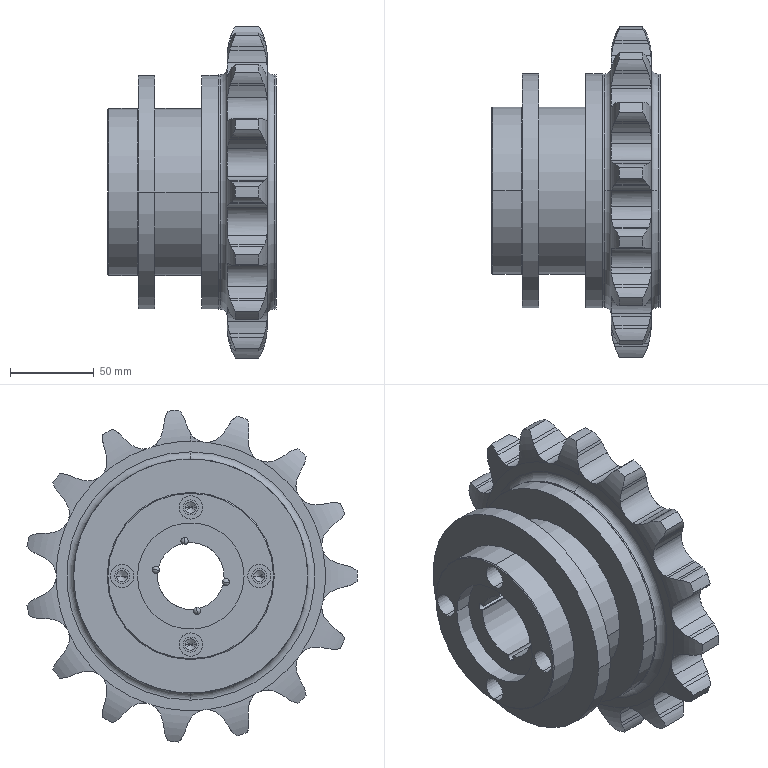Part | SolidWorks | 3 solids | 332 faces | box 100.469 x 197.46 x 198.492 mm | volume 1236352 mm3 | cylinder 185 | plane 51 | sphere 40 | torus 36 | cone 20 | commonest cylinder face diameters 32.838 x32 58.009 x31 22.441 x19 6.8 x16 9 x16 199 x15